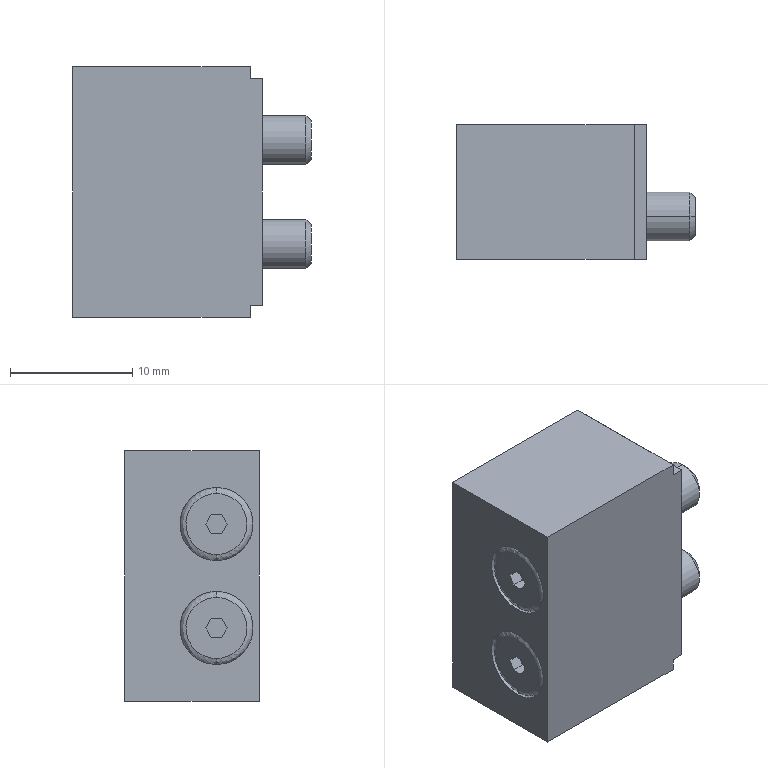Part | STEP file | QA-HI_MDX-12 B | 1 solid | 44 faces | box 19.5 x 11 x 20.5 mm | volume 3566 mm3 | plane 28 | cylinder 8 | spline 4 | cone 4 | commonest cylinder face diameters 4 x4 6 x4